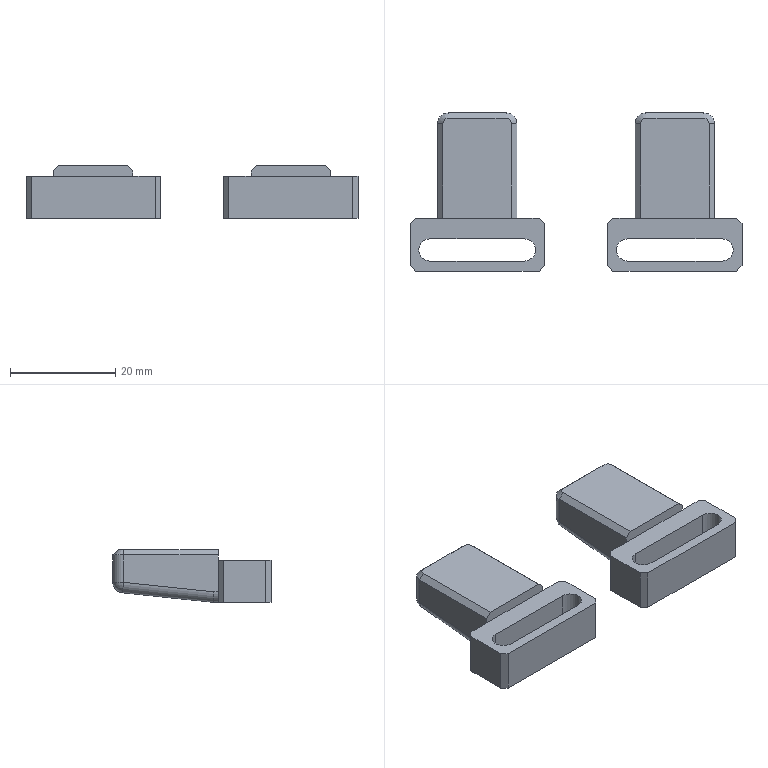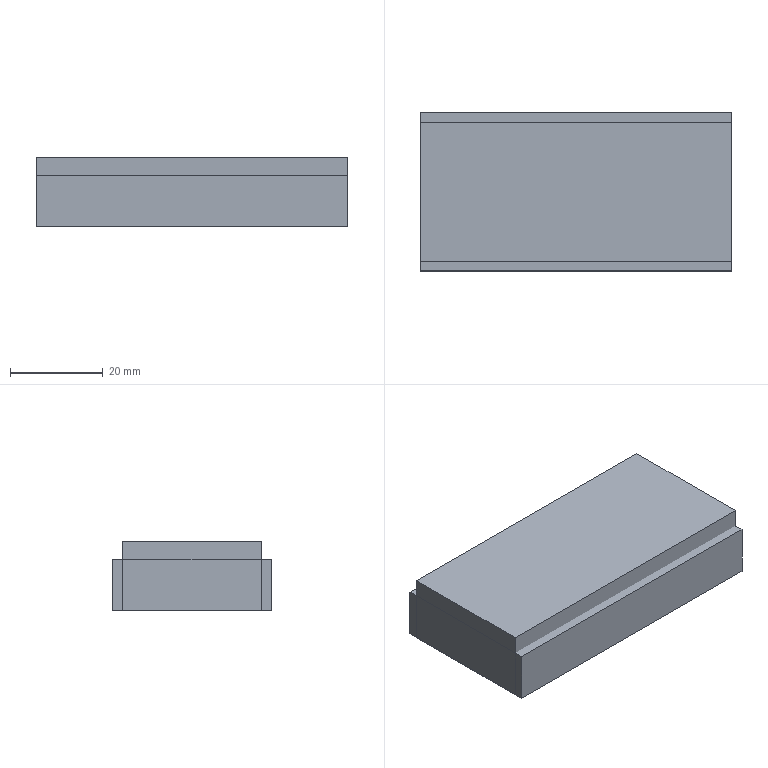CAM job | NX | 3+2 milling | part box 63 x 30 x 10 mm | stock box 67 x 34 x 15 mm
Tools:
number,name,description,diameter,corner_radius,flute_length,length,flutes
19,D80,Milling Tool-5 Parameters,80.0,0.0,50.0,75.0,2
15,D10,Milling Tool-5 Parameters,10.0,0.0,50.0,75.0,2
14,D10JING,Milling Tool-5 Parameters,10.0,0.0,50.0,75.0,2
17,D3,Milling Tool-5 Parameters,3.0,0.0,50.0,75.0,2
1,D6A45,Milling Tool-5 Parameters,6.0,0.0,50.0,75.0,2
16,D4R0.5,Milling Tool-5 Parameters,4.0,0.5,50.0,75.0,2
18,R2,Milling Tool-5 Parameters,4.0,2.0,50.0,75.0,2
6,D6,Milling Tool-5 Parameters,6.0,0.0,50.0,75.0,2
Operations:
program,operation,operation_type,tool,method,geometry_group,spindle_rpm,surface_speed,feed_per_tooth,feed_cut,feed_plunge,cut_length_mm,path_length_mm,cut_time_min,machine_time_min
1,FLOOR_WALL_COPY,VolumeBased25DMillingOperation,D80,METHOD,A,6500.0,1633.0,0.1154,1500.0,100.0,163.0,217.0,0.1087,0.1141
1,ZLEVEL_PROFILE,ZLevelMilling,D10,METHOD,A,9500.0,298.0,0.1579,3000.0,1000.0,2907.355,3108.053,1.033,1.053
1,FLOOR_WALL,VolumeBased25DMillingOperation,D10,METHOD,A,9500.0,298.0,0.1316,2500.0,1000.0,735.82,909.788,0.302,0.3194
1,PLANAR_PROFILE,PlanarMilling,D10,METHOD,A,9500.0,298.0,0.1316,2500.0,1000.0,400.0,474.0,0.226,0.2334
1,ZLEVEL_PROFILE_COPY_1_COPY_COPY_1,ZLevelMilling,D10JING,METHOD,A,9500.0,298.0,0.0632,1200.0,1000.0,283.02,473.166,0.237,0.2561
1,FLOOR_WALL_1,VolumeBased25DMillingOperation,D10JING,METHOD,A,9500.0,119.0,0.0658,1250.0,100.0,479.087,823.974,0.3833,0.4178
1,ZLEVEL_PROFILE_COPY,ZLevelMilling,D3,METHOD,A,9500.0,89.0,0.0632,1200.0,1000.0,2253.304,2417.447,1.889,1.906
1,PLANAR_MILL_COPY_COPY_COPY_COPY_COPY_COPY_1_COPY_1,PlanarMilling,D6A45,METHOD,A,9500.0,179.0,0.0658,1250.0,100.0,157.835,333.535,0.1263,0.1438
1,PLANAR_MILL_COPY_COPY_COPY_COPY_COPY_COPY_1_COPY_1_COPY,PlanarMilling,D6A45,METHOD,A,9500.0,179.0,0.0658,1250.0,100.0,218.478,559.67,0.1748,0.2089
2,FLOOR_WALL_COPY_COPY,VolumeBased25DMillingOperation,D80,METHOD,B,6500.0,1633.0,0.1154,1500.0,100.0,815.0,1691.801,0.5433,0.631
2,FLOOR_WALL_COPY_COPY_COPY,VolumeBased25DMillingOperation,D80,METHOD,B,6500.0,1633.0,0.1154,1500.0,100.0,163.0,217.0,0.1087,0.1141
2,PLANAR_MILL_COPY_COPY_COPY_COPY_COPY_COPY_1_COPY_1_COPY_1,PlanarMilling,D6A45,METHOD,B,9500.0,179.0,0.0658,1250.0,100.0,197.171,469.641,0.1577,0.185
2,FIXED_CONTOUR,SurfaceContour,D4R0.5,METHOD,B,9500.0,119.0,0.1316,2500.0,1000.0,11426.384,11847.74,4.594,4.637
2,FIXED_CONTOUR_COPY,SurfaceContour,R2,METHOD,B,9500.0,119.0,0.1316,2500.0,1000.0,2996.264,3147.627,1.204,1.219
PROGRAM,ZLEVEL_PROFILE_COPY_1_COPY_COPY_1_COPY,ZLevelMilling,D10JING,METHOD,C,9500.0,298.0,0.0632,1200.0,1000.0,136.722,832.054,0.1187,0.1883
PROGRAM,HOLE_MILLING,CylinderMilling,D6,METHOD,C,9500.0,298.0,0.0658,1250.0,100.0,277.274,356.774,0.2218,0.2298